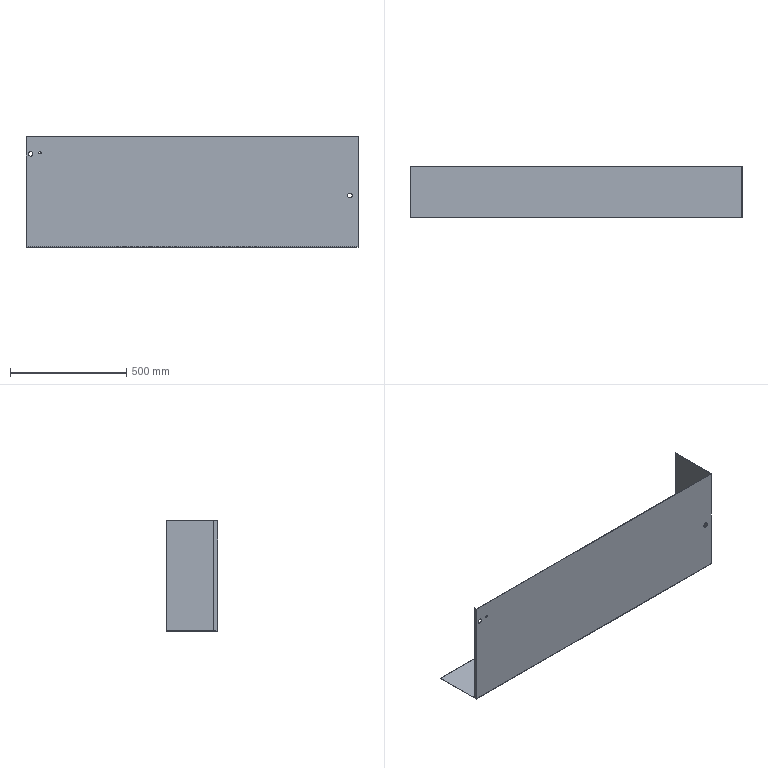Part | 1 solid | 21 faces | box 1430 x 220 x 475 mm | volume 1321657 mm3 | plane 13 | cylinder 8 | commonest cylinder face diameters 20 x4 10 x2 1.473 x1 3.873 x1
STEP:
#1=CARTESIAN_POINT('',(680.,-108.8,230.737));
#2=VERTEX_POINT('',#1);
#3=CARTESIAN_POINT('',(680.,-108.8,210.737));
#4=VERTEX_POINT('',#3);
#5=CARTESIAN_POINT('',(680.,-108.8,220.737));
#6=DIRECTION('',(0.,-1.,0.));
#7=DIRECTION('',(0.,0.,-1.));
#8=AXIS2_PLACEMENT_3D('',#5,#6,#7);
#9=CIRCLE('',#8,10.);
#10=EDGE_CURVE('',#2,#4,#9,.T.);
#11=ORIENTED_EDGE('',*,*,#10,.F.);
#12=CARTESIAN_POINT('',(680.,-110.,230.737));
#13=VERTEX_POINT('',#12);
#14=CARTESIAN_POINT('',(680.,110.,230.737));
#15=DIRECTION('',(0.,-1.,0.));
#16=VECTOR('',#15,1000.);
#17=LINE('',#14,#16);
#18=EDGE_CURVE('',#2,#13,#17,.T.);
#19=ORIENTED_EDGE('',*,*,#18,.T.);
#20=CARTESIAN_POINT('',(680.,-110.,210.737));
#21=VERTEX_POINT('',#20);
#22=CARTESIAN_POINT('',(680.,-110.,220.737));
#23=DIRECTION('',(0.,-1.,0.));
#24=DIRECTION('',(0.,0.,-1.));
#25=AXIS2_PLACEMENT_3D('',#22,#23,#24);
#26=CIRCLE('',#25,10.);
#27=EDGE_CURVE('',#13,#21,#26,.T.);
#28=ORIENTED_EDGE('',*,*,#27,.T.);
#29=CARTESIAN_POINT('',(680.,110.,210.737));
#30=DIRECTION('',(0.,-1.,0.));
#31=VECTOR('',#30,1000.);
#32=LINE('',#29,#31);
#33=EDGE_CURVE('',#4,#21,#32,.T.);
#34=ORIENTED_EDGE('',*,*,#33,.F.);
#35=EDGE_LOOP('',(#11,#19,#28,#34));
#36=FACE_OUTER_BOUND('',#35,.T.);
#37=CARTESIAN_POINT('',(680.,110.,220.737));
#38=DIRECTION('',(0.,-1.,0.));
#39=DIRECTION('',(0.,0.,-1.));
#40=AXIS2_PLACEMENT_3D('',#37,#38,#39);
#41=CYLINDRICAL_SURFACE('',#40,10.);
#42=ADVANCED_FACE('',(#36),#41,.F.);
#43=CARTESIAN_POINT('',(-695.,-108.8,410.737));
#44=VERTEX_POINT('',#43);
#45=CARTESIAN_POINT('',(-695.,-108.8,390.737));
#46=VERTEX_POINT('',#45);
#47=CARTESIAN_POINT('',(-695.,-108.8,400.737));
#48=DIRECTION('',(0.,-1.,0.));
#49=DIRECTION('',(0.,0.,-1.));
#50=AXIS2_PLACEMENT_3D('',#47,#48,#49);
#51=CIRCLE('',#50,10.);
#52=EDGE_CURVE('',#44,#46,#51,.T.);
#53=ORIENTED_EDGE('',*,*,#52,.F.);
#54=CARTESIAN_POINT('',(-695.,-110.,410.737));
#55=VERTEX_POINT('',#54);
#56=CARTESIAN_POINT('',(-695.,110.,410.737));
#57=DIRECTION('',(0.,-1.,0.));
#58=VECTOR('',#57,1000.);
#59=LINE('',#56,#58);
#60=EDGE_CURVE('',#44,#55,#59,.T.);
#61=ORIENTED_EDGE('',*,*,#60,.T.);
#62=CARTESIAN_POINT('',(-695.,-110.,390.737));
#63=VERTEX_POINT('',#62);
#64=CARTESIAN_POINT('',(-695.,-110.,400.737));
#65=DIRECTION('',(0.,-1.,0.));
#66=DIRECTION('',(0.,0.,-1.));
#67=AXIS2_PLACEMENT_3D('',#64,#65,#66);
#68=CIRCLE('',#67,10.);
#69=EDGE_CURVE('',#55,#63,#68,.T.);
#70=ORIENTED_EDGE('',*,*,#69,.T.);
#71=CARTESIAN_POINT('',(-695.,110.,390.737));
#72=DIRECTION('',(0.,-1.,0.));
#73=VECTOR('',#72,1000.);
#74=LINE('',#71,#73);
#75=EDGE_CURVE('',#46,#63,#74,.T.);
#76=ORIENTED_EDGE('',*,*,#75,.F.);
#77=EDGE_LOOP('',(#53,#61,#70,#76));
#78=FACE_OUTER_BOUND('',#77,.T.);
#79=CARTESIAN_POINT('',(-695.,110.,400.737));
#80=DIRECTION('',(0.,-1.,0.));
#81=DIRECTION('',(0.,0.,-1.));
#82=AXIS2_PLACEMENT_3D('',#79,#80,#81);
#83=CYLINDRICAL_SURFACE('',#82,10.);
#84=ADVANCED_FACE('',(#78),#83,.F.);
#85=CARTESIAN_POINT('',(-655.,-108.8,410.737));
#86=VERTEX_POINT('',#85);
#87=CARTESIAN_POINT('',(-655.,-108.8,400.737));
#88=VERTEX_POINT('',#87);
#89=CARTESIAN_POINT('',(-655.,-108.8,405.737));
#90=DIRECTION('',(0.,-1.,0.));
#91=DIRECTION('',(0.,0.,-1.));
#92=AXIS2_PLACEMENT_3D('',#89,#90,#91);
#93=CIRCLE('',#92,5.);
#94=EDGE_CURVE('',#86,#88,#93,.T.);
#95=ORIENTED_EDGE('',*,*,#94,.F.);
#96=CARTESIAN_POINT('',(-655.,-110.,410.737));
#97=VERTEX_POINT('',#96);
#98=CARTESIAN_POINT('',(-655.,110.,410.737));
#99=DIRECTION('',(0.,-1.,0.));
#100=VECTOR('',#99,1000.);
#101=LINE('',#98,#100);
#102=EDGE_CURVE('',#86,#97,#101,.T.);
#103=ORIENTED_EDGE('',*,*,#102,.T.);
#104=CARTESIAN_POINT('',(-655.,-110.,400.737));
#105=VERTEX_POINT('',#104);
#106=CARTESIAN_POINT('',(-655.,-110.,405.737));
#107=DIRECTION('',(0.,-1.,0.));
#108=DIRECTION('',(0.,0.,-1.));
#109=AXIS2_PLACEMENT_3D('',#106,#107,#108);
#110=CIRCLE('',#109,5.);
#111=EDGE_CURVE('',#97,#105,#110,.T.);
#112=ORIENTED_EDGE('',*,*,#111,.T.);
#113=CARTESIAN_POINT('',(-655.,110.,400.737));
#114=DIRECTION('',(0.,-1.,0.));
#115=VECTOR('',#114,1000.);
#116=LINE('',#113,#115);
#117=EDGE_CURVE('',#88,#105,#116,.T.);
#118=ORIENTED_EDGE('',*,*,#117,.F.);
#119=EDGE_LOOP('',(#95,#103,#112,#118));
#120=FACE_OUTER_BOUND('',#119,.T.);
#121=CARTESIAN_POINT('',(-655.,110.,405.737));
#122=DIRECTION('',(0.,-1.,0.));
#123=DIRECTION('',(0.,0.,-1.));
#124=AXIS2_PLACEMENT_3D('',#121,#122,#123);
#125=CYLINDRICAL_SURFACE('',#124,5.);
#126=ADVANCED_FACE('',(#120),#125,.F.);
#127=CARTESIAN_POINT('',(-715.,-93.8,0.));
#128=VERTEX_POINT('',#127);
#129=CARTESIAN_POINT('',(-713.8,-93.8,0.));
#130=VERTEX_POINT('',#129);
#131=CARTESIAN_POINT('',(0.,-93.8,0.));
#132=DIRECTION('',(1.,0.,0.));
#133=VECTOR('',#132,1000.);
#134=LINE('',#131,#133);
#135=EDGE_CURVE('',#128,#130,#134,.T.);
#136=ORIENTED_EDGE('',*,*,#135,.T.);
#137=CARTESIAN_POINT('',(-713.8,-108.063,0.));
#138=VERTEX_POINT('',#137);
#139=CARTESIAN_POINT('',(-713.8,0.,0.));
#140=DIRECTION('',(0.,-1.,0.));
#141=VECTOR('',#140,1000.);
#142=LINE('',#139,#141);
#143=EDGE_CURVE('',#130,#138,#142,.T.);
#144=ORIENTED_EDGE('',*,*,#143,.T.);
#145=CARTESIAN_POINT('',(713.8,-108.063,0.));
#146=VERTEX_POINT('',#145);
#147=CARTESIAN_POINT('',(715.,-108.063,0.));
#148=DIRECTION('',(-1.,0.,0.));
#149=VECTOR('',#148,1000.);
#150=LINE('',#147,#149);
#151=EDGE_CURVE('',#146,#138,#150,.T.);
#152=ORIENTED_EDGE('',*,*,#151,.F.);
#153=CARTESIAN_POINT('',(713.8,110.,0.));
#154=VERTEX_POINT('',#153);
#155=CARTESIAN_POINT('',(713.8,553.802,0.));
#156=DIRECTION('',(0.,-1.,0.));
#157=VECTOR('',#156,1000.);
#158=LINE('',#155,#157);
#159=EDGE_CURVE('',#154,#146,#158,.T.);
#160=ORIENTED_EDGE('',*,*,#159,.F.);
#161=CARTESIAN_POINT('',(-715.,110.,0.));
#162=VERTEX_POINT('',#161);
#163=CARTESIAN_POINT('',(-715.,110.,0.));
#164=DIRECTION('',(-1.,0.,0.));
#165=VECTOR('',#164,1000.);
#166=LINE('',#163,#165);
#167=EDGE_CURVE('',#154,#162,#166,.T.);
#168=ORIENTED_EDGE('',*,*,#167,.T.);
#169=CARTESIAN_POINT('',(-715.,110.,0.));
#170=DIRECTION('',(0.,-1.,0.));
#171=VECTOR('',#170,1000.);
#172=LINE('',#169,#171);
#173=EDGE_CURVE('',#162,#128,#172,.T.);
#174=ORIENTED_EDGE('',*,*,#173,.T.);
#175=EDGE_LOOP('',(#136,#144,#152,#160,#168,#174));
#176=FACE_OUTER_BOUND('',#175,.T.);
#177=CARTESIAN_POINT('',(0.,0.,0.));
#178=DIRECTION('',(0.,0.,1.));
#179=DIRECTION('',(1.,0.,0.));
#180=AXIS2_PLACEMENT_3D('',#177,#178,#179);
#181=PLANE('',#180);
#182=ADVANCED_FACE('',(#176),#181,.T.);
#183=CARTESIAN_POINT('',(-713.8,-108.8,0.7366));
#184=VERTEX_POINT('',#183);
#185=CARTESIAN_POINT('',(-713.8,-108.063,0.7366));
#186=DIRECTION('',(1.,0.,0.));
#187=DIRECTION('',(0.,0.,1.));
#188=AXIS2_PLACEMENT_3D('',#185,#186,#187);
#189=CIRCLE('',#188,0.7366);
#190=EDGE_CURVE('',#184,#138,#189,.T.);
#191=ORIENTED_EDGE('',*,*,#190,.F.);
#192=CARTESIAN_POINT('',(713.8,-108.8,0.7366));
#193=VERTEX_POINT('',#192);
#194=CARTESIAN_POINT('',(-715.,-108.8,0.7366));
#195=DIRECTION('',(1.,0.,0.));
#196=VECTOR('',#195,1000.);
#197=LINE('',#194,#196);
#198=EDGE_CURVE('',#184,#193,#197,.T.);
#199=ORIENTED_EDGE('',*,*,#198,.T.);
#200=CARTESIAN_POINT('',(713.8,-108.063,0.7366));
#201=DIRECTION('',(-1.,0.,0.));
#202=DIRECTION('',(0.,0.,-1.));
#203=AXIS2_PLACEMENT_3D('',#200,#201,#202);
#204=CIRCLE('',#203,0.7366);
#205=EDGE_CURVE('',#146,#193,#204,.T.);
#206=ORIENTED_EDGE('',*,*,#205,.F.);
#207=ORIENTED_EDGE('',*,*,#151,.T.);
#208=EDGE_LOOP('',(#191,#199,#206,#207));
#209=FACE_OUTER_BOUND('',#208,.T.);
#210=CARTESIAN_POINT('',(715.,-108.063,0.7366));
#211=DIRECTION('',(1.,0.,0.));
#212=DIRECTION('',(0.,-1.,0.));
#213=AXIS2_PLACEMENT_3D('',#210,#211,#212);
#214=CYLINDRICAL_SURFACE('',#213,0.7366);
#215=ADVANCED_FACE('',(#209),#214,.F.);
#216=CARTESIAN_POINT('',(-655.,-108.8,405.737));
#217=DIRECTION('',(0.,-1.,0.));
#218=DIRECTION('',(0.,0.,-1.));
#219=AXIS2_PLACEMENT_3D('',#216,#217,#218);
#220=CIRCLE('',#219,5.);
#221=EDGE_CURVE('',#88,#86,#220,.T.);
#222=ORIENTED_EDGE('',*,*,#221,.T.);
#223=ORIENTED_EDGE('',*,*,#94,.T.);
#224=EDGE_LOOP('',(#222,#223));
#225=FACE_BOUND('',#224,.T.);
#226=CARTESIAN_POINT('',(-695.,-108.8,400.737));
#227=DIRECTION('',(0.,-1.,0.));
#228=DIRECTION('',(0.,0.,-1.));
#229=AXIS2_PLACEMENT_3D('',#226,#227,#228);
#230=CIRCLE('',#229,10.);
#231=EDGE_CURVE('',#46,#44,#230,.T.);
#232=ORIENTED_EDGE('',*,*,#231,.T.);
#233=ORIENTED_EDGE('',*,*,#52,.T.);
#234=EDGE_LOOP('',(#232,#233));
#235=FACE_BOUND('',#234,.T.);
#236=CARTESIAN_POINT('',(680.,-108.8,220.737));
#237=DIRECTION('',(0.,-1.,0.));
#238=DIRECTION('',(0.,0.,-1.));
#239=AXIS2_PLACEMENT_3D('',#236,#237,#238);
#240=CIRCLE('',#239,10.);
#241=EDGE_CURVE('',#4,#2,#240,.T.);
#242=ORIENTED_EDGE('',*,*,#241,.T.);
#243=ORIENTED_EDGE('',*,*,#10,.T.);
#244=EDGE_LOOP('',(#242,#243));
#245=FACE_BOUND('',#244,.T.);
#246=CARTESIAN_POINT('',(-713.8,-108.8,473.8));
#247=VERTEX_POINT('',#246);
#248=CARTESIAN_POINT('',(-713.8,-108.8,473.8));
#249=DIRECTION('',(0.,0.,-1.));
#250=VECTOR('',#249,1000.);
#251=LINE('',#248,#250);
#252=EDGE_CURVE('',#247,#184,#251,.T.);
#253=ORIENTED_EDGE('',*,*,#252,.F.);
#254=CARTESIAN_POINT('',(713.8,-108.8,473.8));
#255=VERTEX_POINT('',#254);
#256=CARTESIAN_POINT('',(0.,-108.8,473.8));
#257=DIRECTION('',(1.,0.,0.));
#258=VECTOR('',#257,1000.);
#259=LINE('',#256,#258);
#260=EDGE_CURVE('',#247,#255,#259,.T.);
#261=ORIENTED_EDGE('',*,*,#260,.T.);
#262=CARTESIAN_POINT('',(713.8,-108.8,443.8));
#263=DIRECTION('',(0.,0.,1.));
#264=VECTOR('',#263,1000.);
#265=LINE('',#262,#264);
#266=EDGE_CURVE('',#193,#255,#265,.T.);
#267=ORIENTED_EDGE('',*,*,#266,.F.);
#268=ORIENTED_EDGE('',*,*,#198,.F.);
#269=EDGE_LOOP('',(#253,#261,#267,#268));
#270=FACE_OUTER_BOUND('',#269,.T.);
#271=CARTESIAN_POINT('',(0.,-108.8,0.));
#272=DIRECTION('',(0.,-1.,0.));
#273=DIRECTION('',(0.,0.,-1.));
#274=AXIS2_PLACEMENT_3D('',#271,#272,#273);
#275=PLANE('',#274);
#276=ADVANCED_FACE('',(#225,#235,#245,#270),#275,.F.);
#277=CARTESIAN_POINT('',(-713.8,-108.8,-1.054));
#278=VERTEX_POINT('',#277);
#279=CARTESIAN_POINT('',(-715.,-108.8,-1.054));
#280=VERTEX_POINT('',#279);
#281=CARTESIAN_POINT('',(715.,-108.8,-1.054));
#282=DIRECTION('',(-1.,0.,0.));
#283=VECTOR('',#282,1000.);
#284=LINE('',#281,#283);
#285=EDGE_CURVE('',#278,#280,#284,.T.);
#286=ORIENTED_EDGE('',*,*,#285,.F.);
#287=CARTESIAN_POINT('',(-713.8,-108.063,-1.2));
#288=VERTEX_POINT('',#287);
#289=CARTESIAN_POINT('',(-713.8,-108.063,0.7366));
#290=DIRECTION('',(1.,0.,0.));
#291=DIRECTION('',(0.,0.,1.));
#292=AXIS2_PLACEMENT_3D('',#289,#290,#291);
#293=CIRCLE('',#292,1.937);
#294=EDGE_CURVE('',#278,#288,#293,.T.);
#295=ORIENTED_EDGE('',*,*,#294,.T.);
#296=CARTESIAN_POINT('',(715.,-108.063,-1.2));
#297=VERTEX_POINT('',#296);
#298=CARTESIAN_POINT('',(715.,-108.063,-1.2));
#299=DIRECTION('',(-1.,0.,0.));
#300=VECTOR('',#299,1000.);
#301=LINE('',#298,#300);
#302=EDGE_CURVE('',#297,#288,#301,.T.);
#303=ORIENTED_EDGE('',*,*,#302,.F.);
#304=CARTESIAN_POINT('',(715.,-110.,0.7366));
#305=VERTEX_POINT('',#304);
#306=CARTESIAN_POINT('',(715.,-108.063,0.7366));
#307=DIRECTION('',(1.,0.,0.));
#308=DIRECTION('',(0.,0.,-1.));
#309=AXIS2_PLACEMENT_3D('',#306,#307,#308);
#310=CIRCLE('',#309,1.937);
#311=EDGE_CURVE('',#305,#297,#310,.T.);
#312=ORIENTED_EDGE('',*,*,#311,.F.);
#313=CARTESIAN_POINT('',(-715.,-110.,0.7366));
#314=VERTEX_POINT('',#313);
#315=CARTESIAN_POINT('',(0.,-110.,0.7366));
#316=DIRECTION('',(1.,0.,0.));
#317=VECTOR('',#316,1000.);
#318=LINE('',#315,#317);
#319=EDGE_CURVE('',#314,#305,#318,.T.);
#320=ORIENTED_EDGE('',*,*,#319,.F.);
#321=CARTESIAN_POINT('',(-715.,-108.063,0.7366));
#322=DIRECTION('',(-1.,0.,0.));
#323=DIRECTION('',(0.,0.,-1.));
#324=AXIS2_PLACEMENT_3D('',#321,#322,#323);
#325=CIRCLE('',#324,1.937);
#326=EDGE_CURVE('',#280,#314,#325,.T.);
#327=ORIENTED_EDGE('',*,*,#326,.F.);
#328=EDGE_LOOP('',(#286,#295,#303,#312,#320,#327));
#329=FACE_OUTER_BOUND('',#328,.T.);
#330=CARTESIAN_POINT('',(715.,-108.063,0.7366));
#331=DIRECTION('',(1.,0.,0.));
#332=DIRECTION('',(0.,-1.,0.));
#333=AXIS2_PLACEMENT_3D('',#330,#331,#332);
#334=CYLINDRICAL_SURFACE('',#333,1.937);
#335=ADVANCED_FACE('',(#329),#334,.T.);
#336=ORIENTED_EDGE('',*,*,#311,.T.);
#337=CARTESIAN_POINT('',(715.,110.,-1.2));
#338=VERTEX_POINT('',#337);
#339=CARTESIAN_POINT('',(715.,110.,-1.2));
#340=DIRECTION('',(0.,1.,0.));
#341=VECTOR('',#340,1000.);
#342=LINE('',#339,#341);
#343=EDGE_CURVE('',#297,#338,#342,.T.);
#344=ORIENTED_EDGE('',*,*,#343,.T.);
#345=CARTESIAN_POINT('',(715.,110.,473.8));
#346=VERTEX_POINT('',#345);
#347=CARTESIAN_POINT('',(715.,110.,-1.2));
#348=DIRECTION('',(0.,0.,1.));
#349=VECTOR('',#348,1000.);
#350=LINE('',#347,#349);
#351=EDGE_CURVE('',#338,#346,#350,.T.);
#352=ORIENTED_EDGE('',*,*,#351,.T.);
#353=CARTESIAN_POINT('',(715.,-110.,473.8));
#354=VERTEX_POINT('',#353);
#355=CARTESIAN_POINT('',(715.,-110.,473.8));
#356=DIRECTION('',(0.,1.,0.));
#357=VECTOR('',#356,1000.);
#358=LINE('',#355,#357);
#359=EDGE_CURVE('',#354,#346,#358,.T.);
#360=ORIENTED_EDGE('',*,*,#359,.F.);
#361=CARTESIAN_POINT('',(715.,-110.,0.));
#362=DIRECTION('',(0.,0.,-1.));
#363=VECTOR('',#362,1000.);
#364=LINE('',#361,#363);
#365=EDGE_CURVE('',#354,#305,#364,.T.);
#366=ORIENTED_EDGE('',*,*,#365,.T.);
#367=EDGE_LOOP('',(#336,#344,#352,#360,#366));
#368=FACE_OUTER_BOUND('',#367,.T.);
#369=CARTESIAN_POINT('',(715.,110.,-1.2));
#370=DIRECTION('',(1.,0.,0.));
#371=DIRECTION('',(0.,1.,0.));
#372=AXIS2_PLACEMENT_3D('',#369,#370,#371);
#373=PLANE('',#372);
#374=ADVANCED_FACE('',(#368),#373,.T.);
#375=ORIENTED_EDGE('',*,*,#302,.T.);
#376=CARTESIAN_POINT('',(-713.8,-108.8,-1.2));
#377=VERTEX_POINT('',#376);
#378=CARTESIAN_POINT('',(-713.8,-93.8,-1.2));
#379=DIRECTION('',(0.,-1.,0.));
#380=VECTOR('',#379,1000.);
#381=LINE('',#378,#380);
#382=EDGE_CURVE('',#288,#377,#381,.T.);
#383=ORIENTED_EDGE('',*,*,#382,.T.);
#384=CARTESIAN_POINT('',(-715.,-108.8,-1.2));
#385=VERTEX_POINT('',#384);
#386=CARTESIAN_POINT('',(-715.,-108.8,-1.2));
#387=DIRECTION('',(-1.,0.,0.));
#388=VECTOR('',#387,1000.);
#389=LINE('',#386,#388);
#390=EDGE_CURVE('',#377,#385,#389,.T.);
#391=ORIENTED_EDGE('',*,*,#390,.T.);
#392=CARTESIAN_POINT('',(-715.,110.,-1.2));
#393=VERTEX_POINT('',#392);
#394=CARTESIAN_POINT('',(-715.,110.,-1.2));
#395=DIRECTION('',(0.,-1.,0.));
#396=VECTOR('',#395,1000.);
#397=LINE('',#394,#396);
#398=EDGE_CURVE('',#393,#385,#397,.T.);
#399=ORIENTED_EDGE('',*,*,#398,.F.);
#400=CARTESIAN_POINT('',(-715.,110.,-1.2));
#401=DIRECTION('',(-1.,0.,0.));
#402=VECTOR('',#401,1000.);
#403=LINE('',#400,#402);
#404=EDGE_CURVE('',#338,#393,#403,.T.);
#405=ORIENTED_EDGE('',*,*,#404,.F.);
#406=ORIENTED_EDGE('',*,*,#343,.F.);
#407=EDGE_LOOP('',(#375,#383,#391,#399,#405,#406));
#408=FACE_OUTER_BOUND('',#407,.T.);
#409=CARTESIAN_POINT('',(0.,0.,-1.2));
#410=DIRECTION('',(0.,0.,1.));
#411=DIRECTION('',(1.,0.,0.));
#412=AXIS2_PLACEMENT_3D('',#409,#410,#411);
#413=PLANE('',#412);
#414=ADVANCED_FACE('',(#408),#413,.F.);
#415=ORIENTED_EDGE('',*,*,#326,.T.);
#416=CARTESIAN_POINT('',(-715.,-110.,473.8));
#417=VERTEX_POINT('',#416);
#418=CARTESIAN_POINT('',(-715.,-110.,443.8));
#419=DIRECTION('',(0.,0.,1.));
#420=VECTOR('',#419,1000.);
#421=LINE('',#418,#420);
#422=EDGE_CURVE('',#314,#417,#421,.T.);
#423=ORIENTED_EDGE('',*,*,#422,.T.);
#424=CARTESIAN_POINT('',(-715.,-93.8,473.8));
#425=VERTEX_POINT('',#424);
#426=CARTESIAN_POINT('',(-715.,-110.,473.8));
#427=DIRECTION('',(0.,1.,0.));
#428=VECTOR('',#427,1000.);
#429=LINE('',#426,#428);
#430=EDGE_CURVE('',#417,#425,#429,.T.);
#431=ORIENTED_EDGE('',*,*,#430,.T.);
#432=CARTESIAN_POINT('',(-715.,-93.8,473.8));
#433=DIRECTION('',(0.,0.,1.));
#434=VECTOR('',#433,1000.);
#435=LINE('',#432,#434);
#436=EDGE_CURVE('',#128,#425,#435,.T.);
#437=ORIENTED_EDGE('',*,*,#436,.F.);
#438=ORIENTED_EDGE('',*,*,#173,.F.);
#439=CARTESIAN_POINT('',(-715.,110.,-1.2));
#440=DIRECTION('',(0.,0.,1.));
#441=VECTOR('',#440,1000.);
#442=LINE('',#439,#441);
#443=EDGE_CURVE('',#393,#162,#442,.T.);
#444=ORIENTED_EDGE('',*,*,#443,.F.);
#445=ORIENTED_EDGE('',*,*,#398,.T.);
#446=CARTESIAN_POINT('',(-715.,-108.8,473.8));
#447=DIRECTION('',(0.,0.,1.));
#448=VECTOR('',#447,1000.);
#449=LINE('',#446,#448);
#450=EDGE_CURVE('',#385,#280,#449,.T.);
#451=ORIENTED_EDGE('',*,*,#450,.T.);
#452=EDGE_LOOP('',(#415,#423,#431,#437,#438,#444,#445,#451));
#453=FACE_OUTER_BOUND('',#452,.T.);
#454=CARTESIAN_POINT('',(-715.,110.,-1.2));
#455=DIRECTION('',(-1.,0.,0.));
#456=DIRECTION('',(0.,0.,1.));
#457=AXIS2_PLACEMENT_3D('',#454,#455,#456);
#458=PLANE('',#457);
#459=ADVANCED_FACE('',(#453),#458,.T.);
#460=ORIENTED_EDGE('',*,*,#167,.F.);
#461=CARTESIAN_POINT('',(713.8,110.,473.8));
#462=VERTEX_POINT('',#461);
#463=CARTESIAN_POINT('',(713.8,110.,443.8));
#464=DIRECTION('',(0.,0.,1.));
#465=VECTOR('',#464,1000.);
#466=LINE('',#463,#465);
#467=EDGE_CURVE('',#154,#462,#466,.T.);
#468=ORIENTED_EDGE('',*,*,#467,.T.);
#469=CARTESIAN_POINT('',(715.,110.,473.8));
#470=DIRECTION('',(1.,0.,0.));
#471=VECTOR('',#470,1000.);
#472=LINE('',#469,#471);
#473=EDGE_CURVE('',#462,#346,#472,.T.);
#474=ORIENTED_EDGE('',*,*,#473,.T.);
#475=ORIENTED_EDGE('',*,*,#351,.F.);
#476=ORIENTED_EDGE('',*,*,#404,.T.);
#477=ORIENTED_EDGE('',*,*,#443,.T.);
#478=EDGE_LOOP('',(#460,#468,#474,#475,#476,#477));
#479=FACE_OUTER_BOUND('',#478,.T.);
#480=CARTESIAN_POINT('',(-715.,110.,-1.2));
#481=DIRECTION('',(0.,1.,0.));
#482=DIRECTION('',(0.,0.,1.));
#483=AXIS2_PLACEMENT_3D('',#480,#481,#482);
#484=PLANE('',#483);
#485=ADVANCED_FACE('',(#479),#484,.T.);
#486=CARTESIAN_POINT('',(680.,-110.,220.737));
#487=DIRECTION('',(0.,-1.,0.));
#488=DIRECTION('',(0.,0.,-1.));
#489=AXIS2_PLACEMENT_3D('',#486,#487,#488);
#490=CIRCLE('',#489,10.);
#491=EDGE_CURVE('',#21,#13,#490,.T.);
#492=ORIENTED_EDGE('',*,*,#491,.F.);
#493=ORIENTED_EDGE('',*,*,#27,.F.);
#494=EDGE_LOOP('',(#492,#493));
#495=FACE_BOUND('',#494,.T.);
#496=CARTESIAN_POINT('',(-695.,-110.,400.737));
#497=DIRECTION('',(0.,-1.,0.));
#498=DIRECTION('',(0.,0.,-1.));
#499=AXIS2_PLACEMENT_3D('',#496,#497,#498);
#500=CIRCLE('',#499,10.);
#501=EDGE_CURVE('',#63,#55,#500,.T.);
#502=ORIENTED_EDGE('',*,*,#501,.F.);
#503=ORIENTED_EDGE('',*,*,#69,.F.);
#504=EDGE_LOOP('',(#502,#503));
#505=FACE_BOUND('',#504,.T.);
#506=CARTESIAN_POINT('',(-655.,-110.,405.737));
#507=DIRECTION('',(0.,-1.,0.));
#508=DIRECTION('',(0.,0.,-1.));
#509=AXIS2_PLACEMENT_3D('',#506,#507,#508);
#510=CIRCLE('',#509,5.);
#511=EDGE_CURVE('',#105,#97,#510,.T.);
#512=ORIENTED_EDGE('',*,*,#511,.F.);
#513=ORIENTED_EDGE('',*,*,#111,.F.);
#514=EDGE_LOOP('',(#512,#513));
#515=FACE_BOUND('',#514,.T.);
#516=ORIENTED_EDGE('',*,*,#422,.F.);
#517=ORIENTED_EDGE('',*,*,#319,.T.);
#518=ORIENTED_EDGE('',*,*,#365,.F.);
#519=CARTESIAN_POINT('',(715.,-110.,473.8));
#520=DIRECTION('',(1.,0.,0.));
#521=VECTOR('',#520,1000.);
#522=LINE('',#519,#521);
#523=EDGE_CURVE('',#417,#354,#522,.T.);
#524=ORIENTED_EDGE('',*,*,#523,.F.);
#525=EDGE_LOOP('',(#516,#517,#518,#524));
#526=FACE_OUTER_BOUND('',#525,.T.);
#527=CARTESIAN_POINT('',(0.,-110.,0.));
#528=DIRECTION('',(0.,-1.,0.));
#529=DIRECTION('',(0.,0.,-1.));
#530=AXIS2_PLACEMENT_3D('',#527,#528,#529);
#531=PLANE('',#530);
#532=ADVANCED_FACE('',(#495,#505,#515,#526),#531,.T.);
#533=ORIENTED_EDGE('',*,*,#260,.F.);
#534=CARTESIAN_POINT('',(-713.8,-93.8,473.8));
#535=VERTEX_POINT('',#534);
#536=CARTESIAN_POINT('',(-713.8,-93.8,473.8));
#537=DIRECTION('',(0.,-1.,0.));
#538=VECTOR('',#537,1000.);
#539=LINE('',#536,#538);
#540=EDGE_CURVE('',#535,#247,#539,.T.);
#541=ORIENTED_EDGE('',*,*,#540,.F.);
#542=CARTESIAN_POINT('',(-715.,-93.8,473.8));
#543=DIRECTION('',(1.,0.,0.));
#544=VECTOR('',#543,1000.);
#545=LINE('',#542,#544);
#546=EDGE_CURVE('',#425,#535,#545,.T.);
#547=ORIENTED_EDGE('',*,*,#546,.F.);
#548=ORIENTED_EDGE('',*,*,#430,.F.);
#549=ORIENTED_EDGE('',*,*,#523,.T.);
#550=ORIENTED_EDGE('',*,*,#359,.T.);
#551=ORIENTED_EDGE('',*,*,#473,.F.);
#552=CARTESIAN_POINT('',(713.8,553.802,473.8));
#553=DIRECTION('',(0.,-1.,0.));
#554=VECTOR('',#553,1000.);
#555=LINE('',#552,#554);
#556=EDGE_CURVE('',#462,#255,#555,.T.);
#557=ORIENTED_EDGE('',*,*,#556,.T.);
#558=EDGE_LOOP('',(#533,#541,#547,#548,#549,#550,#551,#557));
#559=FACE_OUTER_BOUND('',#558,.T.);
#560=CARTESIAN_POINT('',(715.,-110.,473.8));
#561=DIRECTION('',(0.,0.,1.));
#562=DIRECTION('',(0.,-1.,0.));
#563=AXIS2_PLACEMENT_3D('',#560,#561,#562);
#564=PLANE('',#563);
#565=ADVANCED_FACE('',(#559),#564,.T.);
#566=ORIENTED_EDGE('',*,*,#159,.T.);
#567=ORIENTED_EDGE('',*,*,#205,.T.);
#568=ORIENTED_EDGE('',*,*,#266,.T.);
#569=ORIENTED_EDGE('',*,*,#556,.F.);
#570=ORIENTED_EDGE('',*,*,#467,.F.);
#571=EDGE_LOOP('',(#566,#567,#568,#569,#570));
#572=FACE_OUTER_BOUND('',#571,.T.);
#573=CARTESIAN_POINT('',(713.8,553.802,443.8));
#574=DIRECTION('',(1.,0.,0.));
#575=DIRECTION('',(0.,0.,-1.));
#576=AXIS2_PLACEMENT_3D('',#573,#574,#575);
#577=PLANE('',#576);
#578=ADVANCED_FACE('',(#572),#577,.F.);
#579=ORIENTED_EDGE('',*,*,#102,.F.);
#580=ORIENTED_EDGE('',*,*,#221,.F.);
#581=ORIENTED_EDGE('',*,*,#117,.T.);
#582=ORIENTED_EDGE('',*,*,#511,.T.);
#583=EDGE_LOOP('',(#579,#580,#581,#582));
#584=FACE_OUTER_BOUND('',#583,.T.);
#585=CARTESIAN_POINT('',(-655.,110.,405.737));
#586=DIRECTION('',(0.,-1.,0.));
#587=DIRECTION('',(0.,0.,-1.));
#588=AXIS2_PLACEMENT_3D('',#585,#586,#587);
#589=CYLINDRICAL_SURFACE('',#588,5.);
#590=ADVANCED_FACE('',(#584),#589,.F.);
#591=ORIENTED_EDGE('',*,*,#60,.F.);
#592=ORIENTED_EDGE('',*,*,#231,.F.);
#593=ORIENTED_EDGE('',*,*,#75,.T.);
#594=ORIENTED_EDGE('',*,*,#501,.T.);
#595=EDGE_LOOP('',(#591,#592,#593,#594));
#596=FACE_OUTER_BOUND('',#595,.T.);
#597=CARTESIAN_POINT('',(-695.,110.,400.737));
#598=DIRECTION('',(0.,-1.,0.));
#599=DIRECTION('',(0.,0.,-1.));
#600=AXIS2_PLACEMENT_3D('',#597,#598,#599);
#601=CYLINDRICAL_SURFACE('',#600,10.);
#602=ADVANCED_FACE('',(#596),#601,.F.);
#603=ORIENTED_EDGE('',*,*,#18,.F.);
#604=ORIENTED_EDGE('',*,*,#241,.F.);
#605=ORIENTED_EDGE('',*,*,#33,.T.);
#606=ORIENTED_EDGE('',*,*,#491,.T.);
#607=EDGE_LOOP('',(#603,#604,#605,#606));
#608=FACE_OUTER_BOUND('',#607,.T.);
#609=CARTESIAN_POINT('',(680.,110.,220.737));
#610=DIRECTION('',(0.,-1.,0.));
#611=DIRECTION('',(0.,0.,-1.));
#612=AXIS2_PLACEMENT_3D('',#609,#610,#611);
#613=CYLINDRICAL_SURFACE('',#612,10.);
#614=ADVANCED_FACE('',(#608),#613,.F.);
#615=ORIENTED_EDGE('',*,*,#143,.F.);
#616=CARTESIAN_POINT('',(-713.8,-93.8,473.8));
#617=DIRECTION('',(0.,0.,-1.));
#618=VECTOR('',#617,1000.);
#619=LINE('',#616,#618);
#620=EDGE_CURVE('',#535,#130,#619,.T.);
#621=ORIENTED_EDGE('',*,*,#620,.F.);
#622=ORIENTED_EDGE('',*,*,#540,.T.);
#623=ORIENTED_EDGE('',*,*,#252,.T.);
#624=ORIENTED_EDGE('',*,*,#190,.T.);
#625=EDGE_LOOP('',(#615,#621,#622,#623,#624));
#626=FACE_OUTER_BOUND('',#625,.T.);
#627=CARTESIAN_POINT('',(-713.8,-93.8,473.8));
#628=DIRECTION('',(-1.,0.,0.));
#629=DIRECTION('',(0.,0.,1.));
#630=AXIS2_PLACEMENT_3D('',#627,#628,#629);
#631=PLANE('',#630);
#632=ADVANCED_FACE('',(#626),#631,.F.);
#633=ORIENTED_EDGE('',*,*,#135,.F.);
#634=ORIENTED_EDGE('',*,*,#436,.T.);
#635=ORIENTED_EDGE('',*,*,#546,.T.);
#636=ORIENTED_EDGE('',*,*,#620,.T.);
#637=EDGE_LOOP('',(#633,#634,#635,#636));
#638=FACE_OUTER_BOUND('',#637,.T.);
#639=CARTESIAN_POINT('',(0.,-93.8,0.));
#640=DIRECTION('',(0.,-1.,0.));
#641=DIRECTION('',(0.,0.,-1.));
#642=AXIS2_PLACEMENT_3D('',#639,#640,#641);
#643=PLANE('',#642);
#644=ADVANCED_FACE('',(#638),#643,.F.);
#645=ORIENTED_EDGE('',*,*,#294,.F.);
#646=CARTESIAN_POINT('',(-713.8,-108.8,473.8));
#647=DIRECTION('',(0.,0.,-1.));
#648=VECTOR('',#647,1000.);
#649=LINE('',#646,#648);
#650=EDGE_CURVE('',#278,#377,#649,.T.);
#651=ORIENTED_EDGE('',*,*,#650,.T.);
#652=ORIENTED_EDGE('',*,*,#382,.F.);
#653=EDGE_LOOP('',(#645,#651,#652));
#654=FACE_OUTER_BOUND('',#653,.T.);
#655=CARTESIAN_POINT('',(-713.8,-93.8,473.8));
#656=DIRECTION('',(-1.,0.,0.));
#657=DIRECTION('',(0.,0.,1.));
#658=AXIS2_PLACEMENT_3D('',#655,#656,#657);
#659=PLANE('',#658);
#660=ADVANCED_FACE('',(#654),#659,.F.);
#661=ORIENTED_EDGE('',*,*,#650,.F.);
#662=ORIENTED_EDGE('',*,*,#285,.T.);
#663=ORIENTED_EDGE('',*,*,#450,.F.);
#664=ORIENTED_EDGE('',*,*,#390,.F.);
#665=EDGE_LOOP('',(#661,#662,#663,#664));
#666=FACE_OUTER_BOUND('',#665,.T.);
#667=CARTESIAN_POINT('',(0.,-108.8,0.));
#668=DIRECTION('',(0.,-1.,0.));
#669=DIRECTION('',(0.,0.,-1.));
#670=AXIS2_PLACEMENT_3D('',#667,#668,#669);
#671=PLANE('',#670);
#672=ADVANCED_FACE('',(#666),#671,.T.);
#673=CLOSED_SHELL('',(#42,#84,#126,#182,#215,#276,#335,#374,#414,#459,#485,#532,#565,#578,#590,#602,#614,#632,#644,#660,#672));
#674=MANIFOLD_SOLID_BREP('',#673);
#675=CARTESIAN_POINT('',(0.,0.,0.));
#676=DIRECTION('',(0.,0.,1.));
#677=DIRECTION('',(1.,0.,0.));
#678=AXIS2_PLACEMENT_3D('',#675,#676,#677);
#679=(LENGTH_UNIT()NAMED_UNIT(*)SI_UNIT(.MILLI.,.METRE.));
#680=UNCERTAINTY_MEASURE_WITH_UNIT(LENGTH_MEASURE(0.00001),#679,'','');
#681=(NAMED_UNIT(*)PLANE_ANGLE_UNIT()SI_UNIT($,.RADIAN.));
#682=(NAMED_UNIT(*)SI_UNIT($,.STERADIAN.)SOLID_ANGLE_UNIT());
#683=(GEOMETRIC_REPRESENTATION_CONTEXT(3)GLOBAL_UNCERTAINTY_ASSIGNED_CONTEXT((#680))GLOBAL_UNIT_ASSIGNED_CONTEXT((#679,#681,#682))REPRESENTATION_CONTEXT('',''));
#684=ADVANCED_BREP_SHAPE_REPRESENTATION('',(#674,#678),#683);